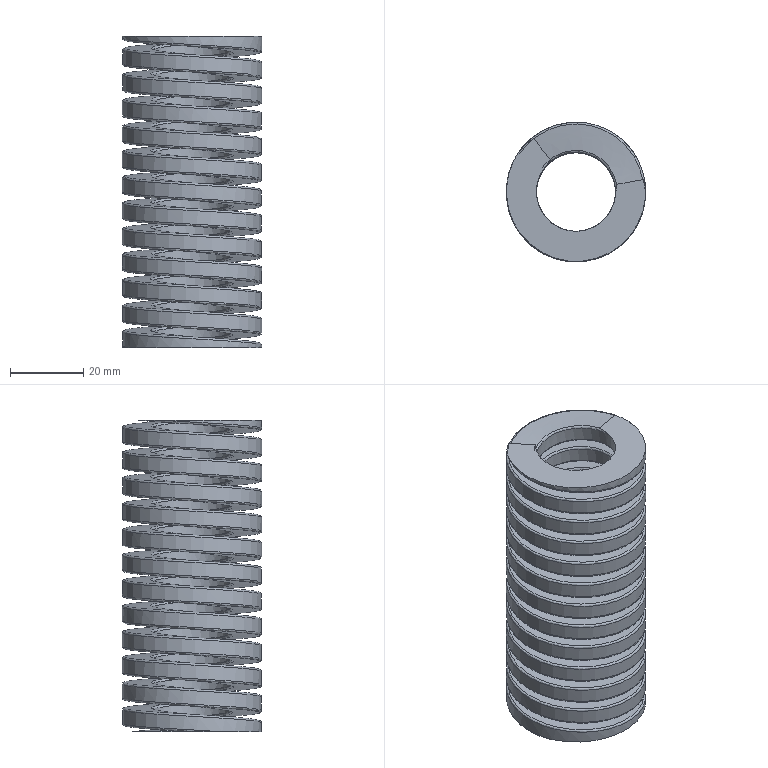Part | STEP file | Mola Vermelha  - R_40-139 - Torre - 1 cav | 1 solid | 10 faces | box 38 x 38 x 85 mm | volume 43568 mm3 | spline 8 | plane 2